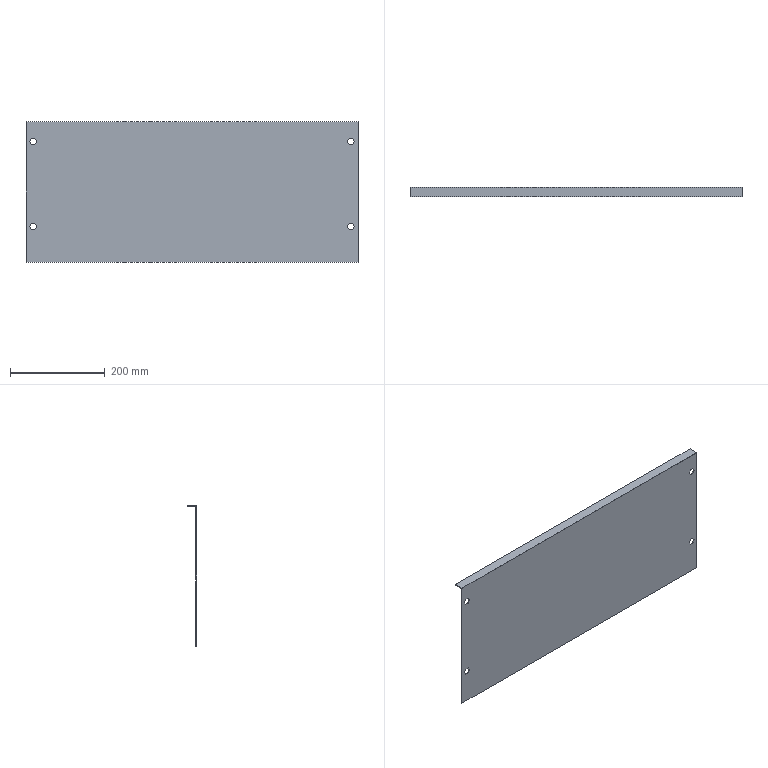Part | SolidWorks | features BaseBody 1 | 1 solid | 32 faces | box 700 x 20 x 297 mm | volume 439829 mm3 | plane 32
STEP:
#1=CARTESIAN_POINT('',(896.946,-3640.973,118.471));
#2=VERTEX_POINT('',#1);
#3=CARTESIAN_POINT('',(896.946,-3640.973,415.471));
#4=VERTEX_POINT('',#3);
#5=CARTESIAN_POINT('',(896.946,-3640.973,415.471));
#6=DIRECTION('',(0.,0.,1.));
#7=VECTOR('',#6,1000.);
#8=LINE('',#5,#7);
#9=EDGE_CURVE('',#2,#4,#8,.T.);
#10=ORIENTED_EDGE('',*,*,#9,.T.);
#11=CARTESIAN_POINT('',(196.946,-3640.973,415.471));
#12=VERTEX_POINT('',#11);
#13=CARTESIAN_POINT('',(896.946,-3640.973,415.471));
#14=DIRECTION('',(-1.,0.,0.));
#15=VECTOR('',#14,1000.);
#16=LINE('',#13,#15);
#17=EDGE_CURVE('',#4,#12,#16,.T.);
#18=ORIENTED_EDGE('',*,*,#17,.T.);
#19=CARTESIAN_POINT('',(196.946,-3640.973,118.471));
#20=VERTEX_POINT('',#19);
#21=CARTESIAN_POINT('',(196.946,-3640.973,415.471));
#22=DIRECTION('',(0.,0.,-1.));
#23=VECTOR('',#22,1000.);
#24=LINE('',#21,#23);
#25=EDGE_CURVE('',#12,#20,#24,.T.);
#26=ORIENTED_EDGE('',*,*,#25,.T.);
#27=CARTESIAN_POINT('',(896.946,-3640.973,118.471));
#28=DIRECTION('',(1.,0.,0.));
#29=VECTOR('',#28,1000.);
#30=LINE('',#27,#29);
#31=EDGE_CURVE('',#20,#2,#30,.T.);
#32=ORIENTED_EDGE('',*,*,#31,.T.);
#33=EDGE_LOOP('',(#10,#18,#26,#32));
#34=FACE_OUTER_BOUND('',#33,.T.);
#35=CARTESIAN_POINT('',(878.193,-3640.973,367.471));
#36=VERTEX_POINT('',#35);
#37=CARTESIAN_POINT('',(874.44,-3640.973,373.971));
#38=VERTEX_POINT('',#37);
#39=CARTESIAN_POINT('',(878.193,-3640.973,367.471));
#40=DIRECTION('',(-0.5,0.,0.866));
#41=VECTOR('',#40,1000.);
#42=LINE('',#39,#41);
#43=EDGE_CURVE('',#36,#38,#42,.T.);
#44=ORIENTED_EDGE('',*,*,#43,.T.);
#45=CARTESIAN_POINT('',(878.193,-3640.973,380.471));
#46=VERTEX_POINT('',#45);
#47=CARTESIAN_POINT('',(874.44,-3640.973,373.971));
#48=DIRECTION('',(0.5,0.,0.866));
#49=VECTOR('',#48,1000.);
#50=LINE('',#47,#49);
#51=EDGE_CURVE('',#38,#46,#50,.T.);
#52=ORIENTED_EDGE('',*,*,#51,.T.);
#53=CARTESIAN_POINT('',(885.698,-3640.973,380.471));
#54=VERTEX_POINT('',#53);
#55=CARTESIAN_POINT('',(896.946,-3640.973,380.471));
#56=DIRECTION('',(1.,0.,0.));
#57=VECTOR('',#56,1000.);
#58=LINE('',#55,#57);
#59=EDGE_CURVE('',#46,#54,#58,.T.);
#60=ORIENTED_EDGE('',*,*,#59,.T.);
#61=CARTESIAN_POINT('',(889.451,-3640.973,373.971));
#62=VERTEX_POINT('',#61);
#63=CARTESIAN_POINT('',(885.698,-3640.973,380.471));
#64=DIRECTION('',(0.5,0.,-0.866));
#65=VECTOR('',#64,1000.);
#66=LINE('',#63,#65);
#67=EDGE_CURVE('',#54,#62,#66,.T.);
#68=ORIENTED_EDGE('',*,*,#67,.T.);
#69=CARTESIAN_POINT('',(885.698,-3640.973,367.471));
#70=VERTEX_POINT('',#69);
#71=CARTESIAN_POINT('',(889.451,-3640.973,373.971));
#72=DIRECTION('',(-0.5,0.,-0.866));
#73=VECTOR('',#72,1000.);
#74=LINE('',#71,#73);
#75=EDGE_CURVE('',#62,#70,#74,.T.);
#76=ORIENTED_EDGE('',*,*,#75,.T.);
#77=CARTESIAN_POINT('',(896.946,-3640.973,367.471));
#78=DIRECTION('',(-1.,0.,0.));
#79=VECTOR('',#78,1000.);
#80=LINE('',#77,#79);
#81=EDGE_CURVE('',#70,#36,#80,.T.);
#82=ORIENTED_EDGE('',*,*,#81,.T.);
#83=EDGE_LOOP('',(#44,#52,#60,#68,#76,#82));
#84=FACE_BOUND('',#83,.T.);
#85=CARTESIAN_POINT('',(208.193,-3640.973,187.471));
#86=VERTEX_POINT('',#85);
#87=CARTESIAN_POINT('',(204.44,-3640.973,193.971));
#88=VERTEX_POINT('',#87);
#89=CARTESIAN_POINT('',(208.193,-3640.973,187.471));
#90=DIRECTION('',(-0.5,0.,0.866));
#91=VECTOR('',#90,1000.);
#92=LINE('',#89,#91);
#93=EDGE_CURVE('',#86,#88,#92,.T.);
#94=ORIENTED_EDGE('',*,*,#93,.T.);
#95=CARTESIAN_POINT('',(208.193,-3640.973,200.471));
#96=VERTEX_POINT('',#95);
#97=CARTESIAN_POINT('',(204.44,-3640.973,193.971));
#98=DIRECTION('',(0.5,0.,0.866));
#99=VECTOR('',#98,1000.);
#100=LINE('',#97,#99);
#101=EDGE_CURVE('',#88,#96,#100,.T.);
#102=ORIENTED_EDGE('',*,*,#101,.T.);
#103=CARTESIAN_POINT('',(215.698,-3640.973,200.471));
#104=VERTEX_POINT('',#103);
#105=CARTESIAN_POINT('',(896.946,-3640.973,200.471));
#106=DIRECTION('',(1.,0.,0.));
#107=VECTOR('',#106,1000.);
#108=LINE('',#105,#107);
#109=EDGE_CURVE('',#96,#104,#108,.T.);
#110=ORIENTED_EDGE('',*,*,#109,.T.);
#111=CARTESIAN_POINT('',(219.451,-3640.973,193.971));
#112=VERTEX_POINT('',#111);
#113=CARTESIAN_POINT('',(215.698,-3640.973,200.471));
#114=DIRECTION('',(0.5,0.,-0.866));
#115=VECTOR('',#114,1000.);
#116=LINE('',#113,#115);
#117=EDGE_CURVE('',#104,#112,#116,.T.);
#118=ORIENTED_EDGE('',*,*,#117,.T.);
#119=CARTESIAN_POINT('',(215.698,-3640.973,187.471));
#120=VERTEX_POINT('',#119);
#121=CARTESIAN_POINT('',(219.451,-3640.973,193.971));
#122=DIRECTION('',(-0.5,0.,-0.866));
#123=VECTOR('',#122,1000.);
#124=LINE('',#121,#123);
#125=EDGE_CURVE('',#112,#120,#124,.T.);
#126=ORIENTED_EDGE('',*,*,#125,.T.);
#127=CARTESIAN_POINT('',(896.946,-3640.973,187.471));
#128=DIRECTION('',(-1.,0.,0.));
#129=VECTOR('',#128,1000.);
#130=LINE('',#127,#129);
#131=EDGE_CURVE('',#120,#86,#130,.T.);
#132=ORIENTED_EDGE('',*,*,#131,.T.);
#133=EDGE_LOOP('',(#94,#102,#110,#118,#126,#132));
#134=FACE_BOUND('',#133,.T.);
#135=CARTESIAN_POINT('',(208.193,-3640.973,367.471));
#136=VERTEX_POINT('',#135);
#137=CARTESIAN_POINT('',(204.44,-3640.973,373.971));
#138=VERTEX_POINT('',#137);
#139=CARTESIAN_POINT('',(208.193,-3640.973,367.471));
#140=DIRECTION('',(-0.5,0.,0.866));
#141=VECTOR('',#140,1000.);
#142=LINE('',#139,#141);
#143=EDGE_CURVE('',#136,#138,#142,.T.);
#144=ORIENTED_EDGE('',*,*,#143,.T.);
#145=CARTESIAN_POINT('',(208.193,-3640.973,380.471));
#146=VERTEX_POINT('',#145);
#147=CARTESIAN_POINT('',(204.44,-3640.973,373.971));
#148=DIRECTION('',(0.5,0.,0.866));
#149=VECTOR('',#148,1000.);
#150=LINE('',#147,#149);
#151=EDGE_CURVE('',#138,#146,#150,.T.);
#152=ORIENTED_EDGE('',*,*,#151,.T.);
#153=CARTESIAN_POINT('',(215.698,-3640.973,380.471));
#154=VERTEX_POINT('',#153);
#155=CARTESIAN_POINT('',(896.946,-3640.973,380.471));
#156=DIRECTION('',(1.,0.,0.));
#157=VECTOR('',#156,1000.);
#158=LINE('',#155,#157);
#159=EDGE_CURVE('',#146,#154,#158,.T.);
#160=ORIENTED_EDGE('',*,*,#159,.T.);
#161=CARTESIAN_POINT('',(219.451,-3640.973,373.971));
#162=VERTEX_POINT('',#161);
#163=CARTESIAN_POINT('',(215.698,-3640.973,380.471));
#164=DIRECTION('',(0.5,0.,-0.866));
#165=VECTOR('',#164,1000.);
#166=LINE('',#163,#165);
#167=EDGE_CURVE('',#154,#162,#166,.T.);
#168=ORIENTED_EDGE('',*,*,#167,.T.);
#169=CARTESIAN_POINT('',(215.698,-3640.973,367.471));
#170=VERTEX_POINT('',#169);
#171=CARTESIAN_POINT('',(219.451,-3640.973,373.971));
#172=DIRECTION('',(-0.5,0.,-0.866));
#173=VECTOR('',#172,1000.);
#174=LINE('',#171,#173);
#175=EDGE_CURVE('',#162,#170,#174,.T.);
#176=ORIENTED_EDGE('',*,*,#175,.T.);
#177=CARTESIAN_POINT('',(896.946,-3640.973,367.471));
#178=DIRECTION('',(-1.,0.,0.));
#179=VECTOR('',#178,1000.);
#180=LINE('',#177,#179);
#181=EDGE_CURVE('',#170,#136,#180,.T.);
#182=ORIENTED_EDGE('',*,*,#181,.T.);
#183=EDGE_LOOP('',(#144,#152,#160,#168,#176,#182));
#184=FACE_BOUND('',#183,.T.);
#185=CARTESIAN_POINT('',(878.193,-3640.973,187.471));
#186=VERTEX_POINT('',#185);
#187=CARTESIAN_POINT('',(874.44,-3640.973,193.971));
#188=VERTEX_POINT('',#187);
#189=CARTESIAN_POINT('',(878.193,-3640.973,187.471));
#190=DIRECTION('',(-0.5,0.,0.866));
#191=VECTOR('',#190,1000.);
#192=LINE('',#189,#191);
#193=EDGE_CURVE('',#186,#188,#192,.T.);
#194=ORIENTED_EDGE('',*,*,#193,.T.);
#195=CARTESIAN_POINT('',(878.193,-3640.973,200.471));
#196=VERTEX_POINT('',#195);
#197=CARTESIAN_POINT('',(874.44,-3640.973,193.971));
#198=DIRECTION('',(0.5,0.,0.866));
#199=VECTOR('',#198,1000.);
#200=LINE('',#197,#199);
#201=EDGE_CURVE('',#188,#196,#200,.T.);
#202=ORIENTED_EDGE('',*,*,#201,.T.);
#203=CARTESIAN_POINT('',(885.698,-3640.973,200.471));
#204=VERTEX_POINT('',#203);
#205=CARTESIAN_POINT('',(896.946,-3640.973,200.471));
#206=DIRECTION('',(1.,0.,0.));
#207=VECTOR('',#206,1000.);
#208=LINE('',#205,#207);
#209=EDGE_CURVE('',#196,#204,#208,.T.);
#210=ORIENTED_EDGE('',*,*,#209,.T.);
#211=CARTESIAN_POINT('',(889.451,-3640.973,193.971));
#212=VERTEX_POINT('',#211);
#213=CARTESIAN_POINT('',(885.698,-3640.973,200.471));
#214=DIRECTION('',(0.5,0.,-0.866));
#215=VECTOR('',#214,1000.);
#216=LINE('',#213,#215);
#217=EDGE_CURVE('',#204,#212,#216,.T.);
#218=ORIENTED_EDGE('',*,*,#217,.T.);
#219=CARTESIAN_POINT('',(885.698,-3640.973,187.471));
#220=VERTEX_POINT('',#219);
#221=CARTESIAN_POINT('',(889.451,-3640.973,193.971));
#222=DIRECTION('',(-0.5,0.,-0.866));
#223=VECTOR('',#222,1000.);
#224=LINE('',#221,#223);
#225=EDGE_CURVE('',#212,#220,#224,.T.);
#226=ORIENTED_EDGE('',*,*,#225,.T.);
#227=CARTESIAN_POINT('',(896.946,-3640.973,187.471));
#228=DIRECTION('',(-1.,0.,0.));
#229=VECTOR('',#228,1000.);
#230=LINE('',#227,#229);
#231=EDGE_CURVE('',#220,#186,#230,.T.);
#232=ORIENTED_EDGE('',*,*,#231,.T.);
#233=EDGE_LOOP('',(#194,#202,#210,#218,#226,#232));
#234=FACE_BOUND('',#233,.T.);
#235=CARTESIAN_POINT('',(896.946,-3640.973,415.471));
#236=DIRECTION('',(0.,-1.,0.));
#237=DIRECTION('',(0.,0.,-1.));
#238=AXIS2_PLACEMENT_3D('',#235,#236,#237);
#239=PLANE('',#238);
#240=ADVANCED_FACE('',(#34,#84,#134,#184,#234),#239,.T.);
#241=CARTESIAN_POINT('',(896.946,-3620.973,415.471));
#242=VERTEX_POINT('',#241);
#243=CARTESIAN_POINT('',(896.946,-3620.973,415.471));
#244=DIRECTION('',(0.,1.,0.));
#245=VECTOR('',#244,1000.);
#246=LINE('',#243,#245);
#247=EDGE_CURVE('',#4,#242,#246,.T.);
#248=ORIENTED_EDGE('',*,*,#247,.T.);
#249=CARTESIAN_POINT('',(196.946,-3620.973,415.471));
#250=VERTEX_POINT('',#249);
#251=CARTESIAN_POINT('',(896.946,-3620.973,415.471));
#252=DIRECTION('',(-1.,0.,0.));
#253=VECTOR('',#252,1000.);
#254=LINE('',#251,#253);
#255=EDGE_CURVE('',#242,#250,#254,.T.);
#256=ORIENTED_EDGE('',*,*,#255,.T.);
#257=CARTESIAN_POINT('',(196.946,-3620.973,415.471));
#258=DIRECTION('',(0.,-1.,0.));
#259=VECTOR('',#258,1000.);
#260=LINE('',#257,#259);
#261=EDGE_CURVE('',#250,#12,#260,.T.);
#262=ORIENTED_EDGE('',*,*,#261,.T.);
#263=ORIENTED_EDGE('',*,*,#17,.F.);
#264=EDGE_LOOP('',(#248,#256,#262,#263));
#265=FACE_OUTER_BOUND('',#264,.T.);
#266=CARTESIAN_POINT('',(896.946,-3620.973,415.471));
#267=DIRECTION('',(0.,0.,1.));
#268=DIRECTION('',(1.,0.,0.));
#269=AXIS2_PLACEMENT_3D('',#266,#267,#268);
#270=PLANE('',#269);
#271=ADVANCED_FACE('',(#265),#270,.T.);
#272=ORIENTED_EDGE('',*,*,#247,.F.);
#273=ORIENTED_EDGE('',*,*,#9,.F.);
#274=CARTESIAN_POINT('',(896.946,-3638.973,118.471));
#275=VERTEX_POINT('',#274);
#276=CARTESIAN_POINT('',(896.946,-3639.349,118.471));
#277=DIRECTION('',(0.,1.,0.));
#278=VECTOR('',#277,1000.);
#279=LINE('',#276,#278);
#280=EDGE_CURVE('',#2,#275,#279,.T.);
#281=ORIENTED_EDGE('',*,*,#280,.T.);
#282=CARTESIAN_POINT('',(896.946,-3638.973,413.471));
#283=VERTEX_POINT('',#282);
#284=CARTESIAN_POINT('',(896.946,-3638.973,275.347));
#285=DIRECTION('',(0.,0.,1.));
#286=VECTOR('',#285,1000.);
#287=LINE('',#284,#286);
#288=EDGE_CURVE('',#275,#283,#287,.T.);
#289=ORIENTED_EDGE('',*,*,#288,.T.);
#290=CARTESIAN_POINT('',(896.946,-3620.973,413.471));
#291=VERTEX_POINT('',#290);
#292=CARTESIAN_POINT('',(896.946,-3639.349,413.471));
#293=DIRECTION('',(0.,1.,0.));
#294=VECTOR('',#293,1000.);
#295=LINE('',#292,#294);
#296=EDGE_CURVE('',#283,#291,#295,.T.);
#297=ORIENTED_EDGE('',*,*,#296,.T.);
#298=CARTESIAN_POINT('',(896.946,-3620.973,275.347));
#299=DIRECTION('',(0.,0.,1.));
#300=VECTOR('',#299,1000.);
#301=LINE('',#298,#300);
#302=EDGE_CURVE('',#291,#242,#301,.T.);
#303=ORIENTED_EDGE('',*,*,#302,.T.);
#304=EDGE_LOOP('',(#272,#273,#281,#289,#297,#303));
#305=FACE_OUTER_BOUND('',#304,.T.);
#306=CARTESIAN_POINT('',(896.946,-3639.349,275.347));
#307=DIRECTION('',(1.,0.,0.));
#308=DIRECTION('',(0.,0.,-1.));
#309=AXIS2_PLACEMENT_3D('',#306,#307,#308);
#310=PLANE('',#309);
#311=ADVANCED_FACE('',(#305),#310,.T.);
#312=ORIENTED_EDGE('',*,*,#280,.F.);
#313=ORIENTED_EDGE('',*,*,#31,.F.);
#314=CARTESIAN_POINT('',(196.946,-3638.973,118.471));
#315=VERTEX_POINT('',#314);
#316=CARTESIAN_POINT('',(196.946,-3640.973,118.471));
#317=DIRECTION('',(0.,1.,0.));
#318=VECTOR('',#317,1000.);
#319=LINE('',#316,#318);
#320=EDGE_CURVE('',#20,#315,#319,.T.);
#321=ORIENTED_EDGE('',*,*,#320,.T.);
#322=CARTESIAN_POINT('',(896.946,-3638.973,118.471));
#323=DIRECTION('',(1.,0.,0.));
#324=VECTOR('',#323,1000.);
#325=LINE('',#322,#324);
#326=EDGE_CURVE('',#315,#275,#325,.T.);
#327=ORIENTED_EDGE('',*,*,#326,.T.);
#328=EDGE_LOOP('',(#312,#313,#321,#327));
#329=FACE_OUTER_BOUND('',#328,.T.);
#330=CARTESIAN_POINT('',(896.946,-3640.973,118.471));
#331=DIRECTION('',(0.,0.,-1.));
#332=DIRECTION('',(-1.,0.,0.));
#333=AXIS2_PLACEMENT_3D('',#330,#331,#332);
#334=PLANE('',#333);
#335=ADVANCED_FACE('',(#329),#334,.T.);
#336=ORIENTED_EDGE('',*,*,#320,.F.);
#337=ORIENTED_EDGE('',*,*,#25,.F.);
#338=ORIENTED_EDGE('',*,*,#261,.F.);
#339=CARTESIAN_POINT('',(196.946,-3620.973,413.471));
#340=VERTEX_POINT('',#339);
#341=CARTESIAN_POINT('',(196.946,-3620.973,275.347));
#342=DIRECTION('',(0.,0.,1.));
#343=VECTOR('',#342,1000.);
#344=LINE('',#341,#343);
#345=EDGE_CURVE('',#340,#250,#344,.T.);
#346=ORIENTED_EDGE('',*,*,#345,.F.);
#347=CARTESIAN_POINT('',(196.946,-3638.973,413.471));
#348=VERTEX_POINT('',#347);
#349=CARTESIAN_POINT('',(196.946,-3639.349,413.471));
#350=DIRECTION('',(0.,1.,0.));
#351=VECTOR('',#350,1000.);
#352=LINE('',#349,#351);
#353=EDGE_CURVE('',#348,#340,#352,.T.);
#354=ORIENTED_EDGE('',*,*,#353,.F.);
#355=CARTESIAN_POINT('',(196.946,-3638.973,275.347));
#356=DIRECTION('',(0.,0.,1.));
#357=VECTOR('',#356,1000.);
#358=LINE('',#355,#357);
#359=EDGE_CURVE('',#315,#348,#358,.T.);
#360=ORIENTED_EDGE('',*,*,#359,.F.);
#361=EDGE_LOOP('',(#336,#337,#338,#346,#354,#360));
#362=FACE_OUTER_BOUND('',#361,.T.);
#363=CARTESIAN_POINT('',(196.946,-3639.349,275.347));
#364=DIRECTION('',(1.,0.,0.));
#365=DIRECTION('',(0.,0.,-1.));
#366=AXIS2_PLACEMENT_3D('',#363,#364,#365);
#367=PLANE('',#366);
#368=ADVANCED_FACE('',(#362),#367,.F.);
#369=CARTESIAN_POINT('',(878.193,-3638.973,380.471));
#370=VERTEX_POINT('',#369);
#371=CARTESIAN_POINT('',(878.193,-3446.271,380.471));
#372=DIRECTION('',(0.,1.,0.));
#373=VECTOR('',#372,1000.);
#374=LINE('',#371,#373);
#375=EDGE_CURVE('',#46,#370,#374,.T.);
#376=ORIENTED_EDGE('',*,*,#375,.F.);
#377=ORIENTED_EDGE('',*,*,#51,.F.);
#378=CARTESIAN_POINT('',(874.44,-3638.973,373.971));
#379=VERTEX_POINT('',#378);
#380=CARTESIAN_POINT('',(874.44,-3446.271,373.971));
#381=DIRECTION('',(0.,-1.,0.));
#382=VECTOR('',#381,1000.);
#383=LINE('',#380,#382);
#384=EDGE_CURVE('',#379,#38,#383,.T.);
#385=ORIENTED_EDGE('',*,*,#384,.F.);
#386=CARTESIAN_POINT('',(878.193,-3638.973,380.471));
#387=DIRECTION('',(-0.5,0.,-0.866));
#388=VECTOR('',#387,1000.);
#389=LINE('',#386,#388);
#390=EDGE_CURVE('',#370,#379,#389,.T.);
#391=ORIENTED_EDGE('',*,*,#390,.F.);
#392=EDGE_LOOP('',(#376,#377,#385,#391));
#393=FACE_OUTER_BOUND('',#392,.T.);
#394=CARTESIAN_POINT('',(878.193,-3446.271,380.471));
#395=DIRECTION('',(-0.866,0.,0.5));
#396=DIRECTION('',(0.5,0.,0.866));
#397=AXIS2_PLACEMENT_3D('',#394,#395,#396);
#398=PLANE('',#397);
#399=ADVANCED_FACE('',(#393),#398,.F.);
#400=ORIENTED_EDGE('',*,*,#384,.T.);
#401=ORIENTED_EDGE('',*,*,#43,.F.);
#402=CARTESIAN_POINT('',(878.193,-3638.973,367.471));
#403=VERTEX_POINT('',#402);
#404=CARTESIAN_POINT('',(878.193,-3446.271,367.471));
#405=DIRECTION('',(0.,-1.,0.));
#406=VECTOR('',#405,1000.);
#407=LINE('',#404,#406);
#408=EDGE_CURVE('',#403,#36,#407,.T.);
#409=ORIENTED_EDGE('',*,*,#408,.F.);
#410=CARTESIAN_POINT('',(874.44,-3638.973,373.971));
#411=DIRECTION('',(0.5,0.,-0.866));
#412=VECTOR('',#411,1000.);
#413=LINE('',#410,#412);
#414=EDGE_CURVE('',#379,#403,#413,.T.);
#415=ORIENTED_EDGE('',*,*,#414,.F.);
#416=EDGE_LOOP('',(#400,#401,#409,#415));
#417=FACE_OUTER_BOUND('',#416,.T.);
#418=CARTESIAN_POINT('',(874.44,-3446.271,373.971));
#419=DIRECTION('',(-0.866,0.,-0.5));
#420=DIRECTION('',(-0.5,0.,0.866));
#421=AXIS2_PLACEMENT_3D('',#418,#419,#420);
#422=PLANE('',#421);
#423=ADVANCED_FACE('',(#417),#422,.F.);
#424=ORIENTED_EDGE('',*,*,#408,.T.);
#425=ORIENTED_EDGE('',*,*,#81,.F.);
#426=CARTESIAN_POINT('',(885.698,-3638.973,367.471));
#427=VERTEX_POINT('',#426);
#428=CARTESIAN_POINT('',(885.698,-3446.271,367.471));
#429=DIRECTION('',(0.,-1.,0.));
#430=VECTOR('',#429,1000.);
#431=LINE('',#428,#430);
#432=EDGE_CURVE('',#427,#70,#431,.T.);
#433=ORIENTED_EDGE('',*,*,#432,.F.);
#434=CARTESIAN_POINT('',(878.193,-3638.973,367.471));
#435=DIRECTION('',(1.,0.,0.));
#436=VECTOR('',#435,1000.);
#437=LINE('',#434,#436);
#438=EDGE_CURVE('',#403,#427,#437,.T.);
#439=ORIENTED_EDGE('',*,*,#438,.F.);
#440=EDGE_LOOP('',(#424,#425,#433,#439));
#441=FACE_OUTER_BOUND('',#440,.T.);
#442=CARTESIAN_POINT('',(878.193,-3446.271,367.471));
#443=DIRECTION('',(0.,0.,-1.));
#444=DIRECTION('',(-1.,0.,0.));
#445=AXIS2_PLACEMENT_3D('',#442,#443,#444);
#446=PLANE('',#445);
#447=ADVANCED_FACE('',(#441),#446,.F.);
#448=ORIENTED_EDGE('',*,*,#432,.T.);
#449=ORIENTED_EDGE('',*,*,#75,.F.);
#450=CARTESIAN_POINT('',(889.451,-3638.973,373.971));
#451=VERTEX_POINT('',#450);
#452=CARTESIAN_POINT('',(889.451,-3446.271,373.971));
#453=DIRECTION('',(0.,-1.,0.));
#454=VECTOR('',#453,1000.);
#455=LINE('',#452,#454);
#456=EDGE_CURVE('',#451,#62,#455,.T.);
#457=ORIENTED_EDGE('',*,*,#456,.F.);
#458=CARTESIAN_POINT('',(885.698,-3638.973,367.471));
#459=DIRECTION('',(0.5,0.,0.866));
#460=VECTOR('',#459,1000.);
#461=LINE('',#458,#460);
#462=EDGE_CURVE('',#427,#451,#461,.T.);
#463=ORIENTED_EDGE('',*,*,#462,.F.);
#464=EDGE_LOOP('',(#448,#449,#457,#463));
#465=FACE_OUTER_BOUND('',#464,.T.);
#466=CARTESIAN_POINT('',(885.698,-3446.271,367.471));
#467=DIRECTION('',(0.866,0.,-0.5));
#468=DIRECTION('',(-0.5,0.,-0.866));
#469=AXIS2_PLACEMENT_3D('',#466,#467,#468);
#470=PLANE('',#469);
#471=ADVANCED_FACE('',(#465),#470,.F.);
#472=ORIENTED_EDGE('',*,*,#456,.T.);
#473=ORIENTED_EDGE('',*,*,#67,.F.);
#474=CARTESIAN_POINT('',(885.698,-3638.973,380.471));
#475=VERTEX_POINT('',#474);
#476=CARTESIAN_POINT('',(885.698,-3446.271,380.471));
#477=DIRECTION('',(0.,-1.,0.));
#478=VECTOR('',#477,1000.);
#479=LINE('',#476,#478);
#480=EDGE_CURVE('',#475,#54,#479,.T.);
#481=ORIENTED_EDGE('',*,*,#480,.F.);
#482=CARTESIAN_POINT('',(889.451,-3638.973,373.971));
#483=DIRECTION('',(-0.5,0.,0.866));
#484=VECTOR('',#483,1000.);
#485=LINE('',#482,#484);
#486=EDGE_CURVE('',#451,#475,#485,.T.);
#487=ORIENTED_EDGE('',*,*,#486,.F.);
#488=EDGE_LOOP('',(#472,#473,#481,#487));
#489=FACE_OUTER_BOUND('',#488,.T.);
#490=CARTESIAN_POINT('',(889.451,-3446.271,373.971));
#491=DIRECTION('',(0.866,0.,0.5));
#492=DIRECTION('',(0.5,0.,-0.866));
#493=AXIS2_PLACEMENT_3D('',#490,#491,#492);
#494=PLANE('',#493);
#495=ADVANCED_FACE('',(#489),#494,.F.);
#496=ORIENTED_EDGE('',*,*,#480,.T.);
#497=ORIENTED_EDGE('',*,*,#59,.F.);
#498=ORIENTED_EDGE('',*,*,#375,.T.);
#499=CARTESIAN_POINT('',(885.698,-3638.973,380.471));
#500=DIRECTION('',(-1.,0.,0.));
#501=VECTOR('',#500,1000.);
#502=LINE('',#499,#501);
#503=EDGE_CURVE('',#475,#370,#502,.T.);
#504=ORIENTED_EDGE('',*,*,#503,.F.);
#505=EDGE_LOOP('',(#496,#497,#498,#504));
#506=FACE_OUTER_BOUND('',#505,.T.);
#507=CARTESIAN_POINT('',(885.698,-3446.271,380.471));
#508=DIRECTION('',(0.,0.,1.));
#509=DIRECTION('',(1.,0.,0.));
#510=AXIS2_PLACEMENT_3D('',#507,#508,#509);
#511=PLANE('',#510);
#512=ADVANCED_FACE('',(#506),#511,.F.);
#513=CARTESIAN_POINT('',(208.193,-3638.973,200.471));
#514=VERTEX_POINT('',#513);
#515=CARTESIAN_POINT('',(208.193,-3446.271,200.471));
#516=DIRECTION('',(0.,1.,0.));
#517=VECTOR('',#516,1000.);
#518=LINE('',#515,#517);
#519=EDGE_CURVE('',#96,#514,#518,.T.);
#520=ORIENTED_EDGE('',*,*,#519,.F.);
#521=ORIENTED_EDGE('',*,*,#101,.F.);
#522=CARTESIAN_POINT('',(204.44,-3638.973,193.971));
#523=VERTEX_POINT('',#522);
#524=CARTESIAN_POINT('',(204.44,-3446.271,193.971));
#525=DIRECTION('',(0.,-1.,0.));
#526=VECTOR('',#525,1000.);
#527=LINE('',#524,#526);
#528=EDGE_CURVE('',#523,#88,#527,.T.);
#529=ORIENTED_EDGE('',*,*,#528,.F.);
#530=CARTESIAN_POINT('',(204.44,-3638.973,193.971));
#531=DIRECTION('',(-0.5,0.,-0.866));
#532=VECTOR('',#531,1000.);
#533=LINE('',#530,#532);
#534=EDGE_CURVE('',#514,#523,#533,.T.);
#535=ORIENTED_EDGE('',*,*,#534,.F.);
#536=EDGE_LOOP('',(#520,#521,#529,#535));
#537=FACE_OUTER_BOUND('',#536,.T.);
#538=CARTESIAN_POINT('',(204.44,-3446.271,193.971));
#539=DIRECTION('',(-0.866,0.,0.5));
#540=DIRECTION('',(0.5,0.,0.866));
#541=AXIS2_PLACEMENT_3D('',#538,#539,#540);
#542=PLANE('',#541);
#543=ADVANCED_FACE('',(#537),#542,.F.);
#544=ORIENTED_EDGE('',*,*,#528,.T.);
#545=ORIENTED_EDGE('',*,*,#93,.F.);
#546=CARTESIAN_POINT('',(208.193,-3638.973,187.471));
#547=VERTEX_POINT('',#546);
#548=CARTESIAN_POINT('',(208.193,-3446.271,187.471));
#549=DIRECTION('',(0.,-1.,0.));
#550=VECTOR('',#549,1000.);
#551=LINE('',#548,#550);
#552=EDGE_CURVE('',#547,#86,#551,.T.);
#553=ORIENTED_EDGE('',*,*,#552,.F.);
#554=CARTESIAN_POINT('',(208.193,-3638.973,187.471));
#555=DIRECTION('',(0.5,0.,-0.866));
#556=VECTOR('',#555,1000.);
#557=LINE('',#554,#556);
#558=EDGE_CURVE('',#523,#547,#557,.T.);
#559=ORIENTED_EDGE('',*,*,#558,.F.);
#560=EDGE_LOOP('',(#544,#545,#553,#559));
#561=FACE_OUTER_BOUND('',#560,.T.);
#562=CARTESIAN_POINT('',(208.193,-3446.271,187.471));
#563=DIRECTION('',(-0.866,0.,-0.5));
#564=DIRECTION('',(-0.5,0.,0.866));
#565=AXIS2_PLACEMENT_3D('',#562,#563,#564);
#566=PLANE('',#565);
#567=ADVANCED_FACE('',(#561),#566,.F.);
#568=ORIENTED_EDGE('',*,*,#552,.T.);
#569=ORIENTED_EDGE('',*,*,#131,.F.);
#570=CARTESIAN_POINT('',(215.698,-3638.973,187.471));
#571=VERTEX_POINT('',#570);
#572=CARTESIAN_POINT('',(215.698,-3446.271,187.471));
#573=DIRECTION('',(0.,-1.,0.));
#574=VECTOR('',#573,1000.);
#575=LINE('',#572,#574);
#576=EDGE_CURVE('',#571,#120,#575,.T.);
#577=ORIENTED_EDGE('',*,*,#576,.F.);
#578=CARTESIAN_POINT('',(215.698,-3638.973,187.471));
#579=DIRECTION('',(1.,0.,0.));
#580=VECTOR('',#579,1000.);
#581=LINE('',#578,#580);
#582=EDGE_CURVE('',#547,#571,#581,.T.);
#583=ORIENTED_EDGE('',*,*,#582,.F.);
#584=EDGE_LOOP('',(#568,#569,#577,#583));
#585=FACE_OUTER_BOUND('',#584,.T.);
#586=CARTESIAN_POINT('',(215.698,-3446.271,187.471));
#587=DIRECTION('',(0.,0.,-1.));
#588=DIRECTION('',(-1.,0.,0.));
#589=AXIS2_PLACEMENT_3D('',#586,#587,#588);
#590=PLANE('',#589);
#591=ADVANCED_FACE('',(#585),#590,.F.);
#592=ORIENTED_EDGE('',*,*,#576,.T.);
#593=ORIENTED_EDGE('',*,*,#125,.F.);
#594=CARTESIAN_POINT('',(219.451,-3638.973,193.971));
#595=VERTEX_POINT('',#594);
#596=CARTESIAN_POINT('',(219.451,-3446.271,193.971));
#597=DIRECTION('',(0.,-1.,0.));
#598=VECTOR('',#597,1000.);
#599=LINE('',#596,#598);
#600=EDGE_CURVE('',#595,#112,#599,.T.);
#601=ORIENTED_EDGE('',*,*,#600,.F.);
#602=CARTESIAN_POINT('',(219.451,-3638.973,193.971));
#603=DIRECTION('',(0.5,0.,0.866));
#604=VECTOR('',#603,1000.);
#605=LINE('',#602,#604);
#606=EDGE_CURVE('',#571,#595,#605,.T.);
#607=ORIENTED_EDGE('',*,*,#606,.F.);
#608=EDGE_LOOP('',(#592,#593,#601,#607));
#609=FACE_OUTER_BOUND('',#608,.T.);
#610=CARTESIAN_POINT('',(219.451,-3446.271,193.971));
#611=DIRECTION('',(0.866,0.,-0.5));
#612=DIRECTION('',(-0.5,0.,-0.866));
#613=AXIS2_PLACEMENT_3D('',#610,#611,#612);
#614=PLANE('',#613);
#615=ADVANCED_FACE('',(#609),#614,.F.);
#616=ORIENTED_EDGE('',*,*,#600,.T.);
#617=ORIENTED_EDGE('',*,*,#117,.F.);
#618=CARTESIAN_POINT('',(215.698,-3638.973,200.471));
#619=VERTEX_POINT('',#618);
#620=CARTESIAN_POINT('',(215.698,-3446.271,200.471));
#621=DIRECTION('',(0.,-1.,0.));
#622=VECTOR('',#621,1000.);
#623=LINE('',#620,#622);
#624=EDGE_CURVE('',#619,#104,#623,.T.);
#625=ORIENTED_EDGE('',*,*,#624,.F.);
#626=CARTESIAN_POINT('',(215.698,-3638.973,200.471));
#627=DIRECTION('',(-0.5,0.,0.866));
#628=VECTOR('',#627,1000.);
#629=LINE('',#626,#628);
#630=EDGE_CURVE('',#595,#619,#629,.T.);
#631=ORIENTED_EDGE('',*,*,#630,.F.);
#632=EDGE_LOOP('',(#616,#617,#625,#631));
#633=FACE_OUTER_BOUND('',#632,.T.);
#634=CARTESIAN_POINT('',(215.698,-3446.271,200.471));
#635=DIRECTION('',(0.866,0.,0.5));
#636=DIRECTION('',(0.5,0.,-0.866));
#637=AXIS2_PLACEMENT_3D('',#634,#635,#636);
#638=PLANE('',#637);
#639=ADVANCED_FACE('',(#633),#638,.F.);
#640=ORIENTED_EDGE('',*,*,#624,.T.);
#641=ORIENTED_EDGE('',*,*,#109,.F.);
#642=ORIENTED_EDGE('',*,*,#519,.T.);
#643=CARTESIAN_POINT('',(208.193,-3638.973,200.471));
#644=DIRECTION('',(-1.,0.,0.));
#645=VECTOR('',#644,1000.);
#646=LINE('',#643,#645);
#647=EDGE_CURVE('',#619,#514,#646,.T.);
#648=ORIENTED_EDGE('',*,*,#647,.F.);
#649=EDGE_LOOP('',(#640,#641,#642,#648));
#650=FACE_OUTER_BOUND('',#649,.T.);
#651=CARTESIAN_POINT('',(208.193,-3446.271,200.471));
#652=DIRECTION('',(0.,0.,1.));
#653=DIRECTION('',(1.,0.,0.));
#654=AXIS2_PLACEMENT_3D('',#651,#652,#653);
#655=PLANE('',#654);
#656=ADVANCED_FACE('',(#650),#655,.F.);
#657=CARTESIAN_POINT('',(208.193,-3638.973,380.471));
#658=VERTEX_POINT('',#657);
#659=CARTESIAN_POINT('',(208.193,-3446.271,380.471));
#660=DIRECTION('',(0.,1.,0.));
#661=VECTOR('',#660,1000.);
#662=LINE('',#659,#661);
#663=EDGE_CURVE('',#146,#658,#662,.T.);
#664=ORIENTED_EDGE('',*,*,#663,.F.);
#665=ORIENTED_EDGE('',*,*,#151,.F.);
#666=CARTESIAN_POINT('',(204.44,-3638.973,373.971));
#667=VERTEX_POINT('',#666);
#668=CARTESIAN_POINT('',(204.44,-3446.271,373.971));
#669=DIRECTION('',(0.,-1.,0.));
#670=VECTOR('',#669,1000.);
#671=LINE('',#668,#670);
#672=EDGE_CURVE('',#667,#138,#671,.T.);
#673=ORIENTED_EDGE('',*,*,#672,.F.);
#674=CARTESIAN_POINT('',(204.44,-3638.973,373.971));
#675=DIRECTION('',(-0.5,0.,-0.866));
#676=VECTOR('',#675,1000.);
#677=LINE('',#674,#676);
#678=EDGE_CURVE('',#658,#667,#677,.T.);
#679=ORIENTED_EDGE('',*,*,#678,.F.);
#680=EDGE_LOOP('',(#664,#665,#673,#679));
#681=FACE_OUTER_BOUND('',#680,.T.);
#682=CARTESIAN_POINT('',(204.44,-3446.271,373.971));
#683=DIRECTION('',(-0.866,0.,0.5));
#684=DIRECTION('',(0.5,0.,0.866));
#685=AXIS2_PLACEMENT_3D('',#682,#683,#684);
#686=PLANE('',#685);
#687=ADVANCED_FACE('',(#681),#686,.F.);
#688=ORIENTED_EDGE('',*,*,#672,.T.);
#689=ORIENTED_EDGE('',*,*,#143,.F.);
#690=CARTESIAN_POINT('',(208.193,-3638.973,367.471));
#691=VERTEX_POINT('',#690);
#692=CARTESIAN_POINT('',(208.193,-3446.271,367.471));
#693=DIRECTION('',(0.,-1.,0.));
#694=VECTOR('',#693,1000.);
#695=LINE('',#692,#694);
#696=EDGE_CURVE('',#691,#136,#695,.T.);
#697=ORIENTED_EDGE('',*,*,#696,.F.);
#698=CARTESIAN_POINT('',(208.193,-3638.973,367.471));
#699=DIRECTION('',(0.5,0.,-0.866));
#700=VECTOR('',#699,1000.);
#701=LINE('',#698,#700);
#702=EDGE_CURVE('',#667,#691,#701,.T.);
#703=ORIENTED_EDGE('',*,*,#702,.F.);
#704=EDGE_LOOP('',(#688,#689,#697,#703));
#705=FACE_OUTER_BOUND('',#704,.T.);
#706=CARTESIAN_POINT('',(208.193,-3446.271,367.471));
#707=DIRECTION('',(-0.866,0.,-0.5));
#708=DIRECTION('',(-0.5,0.,0.866));
#709=AXIS2_PLACEMENT_3D('',#706,#707,#708);
#710=PLANE('',#709);
#711=ADVANCED_FACE('',(#705),#710,.F.);
#712=ORIENTED_EDGE('',*,*,#696,.T.);
#713=ORIENTED_EDGE('',*,*,#181,.F.);
#714=CARTESIAN_POINT('',(215.698,-3638.973,367.471));
#715=VERTEX_POINT('',#714);
#716=CARTESIAN_POINT('',(215.698,-3446.271,367.471));
#717=DIRECTION('',(0.,-1.,0.));
#718=VECTOR('',#717,1000.);
#719=LINE('',#716,#718);
#720=EDGE_CURVE('',#715,#170,#719,.T.);
#721=ORIENTED_EDGE('',*,*,#720,.F.);
#722=CARTESIAN_POINT('',(215.698,-3638.973,367.471));
#723=DIRECTION('',(1.,0.,0.));
#724=VECTOR('',#723,1000.);
#725=LINE('',#722,#724);
#726=EDGE_CURVE('',#691,#715,#725,.T.);
#727=ORIENTED_EDGE('',*,*,#726,.F.);
#728=EDGE_LOOP('',(#712,#713,#721,#727));
#729=FACE_OUTER_BOUND('',#728,.T.);
#730=CARTESIAN_POINT('',(215.698,-3446.271,367.471));
#731=DIRECTION('',(0.,0.,-1.));
#732=DIRECTION('',(-1.,0.,0.));
#733=AXIS2_PLACEMENT_3D('',#730,#731,#732);
#734=PLANE('',#733);
#735=ADVANCED_FACE('',(#729),#734,.F.);
#736=ORIENTED_EDGE('',*,*,#720,.T.);
#737=ORIENTED_EDGE('',*,*,#175,.F.);
#738=CARTESIAN_POINT('',(219.451,-3638.973,373.971));
#739=VERTEX_POINT('',#738);
#740=CARTESIAN_POINT('',(219.451,-3446.271,373.971));
#741=DIRECTION('',(0.,-1.,0.));
#742=VECTOR('',#741,1000.);
#743=LINE('',#740,#742);
#744=EDGE_CURVE('',#739,#162,#743,.T.);
#745=ORIENTED_EDGE('',*,*,#744,.F.);
#746=CARTESIAN_POINT('',(219.451,-3638.973,373.971));
#747=DIRECTION('',(0.5,0.,0.866));
#748=VECTOR('',#747,1000.);
#749=LINE('',#746,#748);
#750=EDGE_CURVE('',#715,#739,#749,.T.);
#751=ORIENTED_EDGE('',*,*,#750,.F.);
#752=EDGE_LOOP('',(#736,#737,#745,#751));
#753=FACE_OUTER_BOUND('',#752,.T.);
#754=CARTESIAN_POINT('',(219.451,-3446.271,373.971));
#755=DIRECTION('',(0.866,0.,-0.5));
#756=DIRECTION('',(-0.5,0.,-0.866));
#757=AXIS2_PLACEMENT_3D('',#754,#755,#756);
#758=PLANE('',#757);
#759=ADVANCED_FACE('',(#753),#758,.F.);
#760=ORIENTED_EDGE('',*,*,#744,.T.);
#761=ORIENTED_EDGE('',*,*,#167,.F.);
#762=CARTESIAN_POINT('',(215.698,-3638.973,380.471));
#763=VERTEX_POINT('',#762);
#764=CARTESIAN_POINT('',(215.698,-3446.271,380.471));
#765=DIRECTION('',(0.,-1.,0.));
#766=VECTOR('',#765,1000.);
#767=LINE('',#764,#766);
#768=EDGE_CURVE('',#763,#154,#767,.T.);
#769=ORIENTED_EDGE('',*,*,#768,.F.);
#770=CARTESIAN_POINT('',(215.698,-3638.973,380.471));
#771=DIRECTION('',(-0.5,0.,0.866));
#772=VECTOR('',#771,1000.);
#773=LINE('',#770,#772);
#774=EDGE_CURVE('',#739,#763,#773,.T.);
#775=ORIENTED_EDGE('',*,*,#774,.F.);
#776=EDGE_LOOP('',(#760,#761,#769,#775));
#777=FACE_OUTER_BOUND('',#776,.T.);
#778=CARTESIAN_POINT('',(215.698,-3446.271,380.471));
#779=DIRECTION('',(0.866,0.,0.5));
#780=DIRECTION('',(0.5,0.,-0.866));
#781=AXIS2_PLACEMENT_3D('',#778,#779,#780);
#782=PLANE('',#781);
#783=ADVANCED_FACE('',(#777),#782,.F.);
#784=ORIENTED_EDGE('',*,*,#768,.T.);
#785=ORIENTED_EDGE('',*,*,#159,.F.);
#786=ORIENTED_EDGE('',*,*,#663,.T.);
#787=CARTESIAN_POINT('',(208.193,-3638.973,380.471));
#788=DIRECTION('',(-1.,0.,0.));
#789=VECTOR('',#788,1000.);
#790=LINE('',#787,#789);
#791=EDGE_CURVE('',#763,#658,#790,.T.);
#792=ORIENTED_EDGE('',*,*,#791,.F.);
#793=EDGE_LOOP('',(#784,#785,#786,#792));
#794=FACE_OUTER_BOUND('',#793,.T.);
#795=CARTESIAN_POINT('',(208.193,-3446.271,380.471));
#796=DIRECTION('',(0.,0.,1.));
#797=DIRECTION('',(1.,0.,0.));
#798=AXIS2_PLACEMENT_3D('',#795,#796,#797);
#799=PLANE('',#798);
#800=ADVANCED_FACE('',(#794),#799,.F.);
#801=CARTESIAN_POINT('',(878.193,-3638.973,200.471));
#802=VERTEX_POINT('',#801);
#803=CARTESIAN_POINT('',(878.193,-3446.271,200.471));
#804=DIRECTION('',(0.,1.,0.));
#805=VECTOR('',#804,1000.);
#806=LINE('',#803,#805);
#807=EDGE_CURVE('',#196,#802,#806,.T.);
#808=ORIENTED_EDGE('',*,*,#807,.F.);
#809=ORIENTED_EDGE('',*,*,#201,.F.);
#810=CARTESIAN_POINT('',(874.44,-3638.973,193.971));
#811=VERTEX_POINT('',#810);
#812=CARTESIAN_POINT('',(874.44,-3446.271,193.971));
#813=DIRECTION('',(0.,-1.,0.));
#814=VECTOR('',#813,1000.);
#815=LINE('',#812,#814);
#816=EDGE_CURVE('',#811,#188,#815,.T.);
#817=ORIENTED_EDGE('',*,*,#816,.F.);
#818=CARTESIAN_POINT('',(878.193,-3638.973,200.471));
#819=DIRECTION('',(-0.5,0.,-0.866));
#820=VECTOR('',#819,1000.);
#821=LINE('',#818,#820);
#822=EDGE_CURVE('',#802,#811,#821,.T.);
#823=ORIENTED_EDGE('',*,*,#822,.F.);
#824=EDGE_LOOP('',(#808,#809,#817,#823));
#825=FACE_OUTER_BOUND('',#824,.T.);
#826=CARTESIAN_POINT('',(878.193,-3446.271,200.471));
#827=DIRECTION('',(-0.866,0.,0.5));
#828=DIRECTION('',(0.5,0.,0.866));
#829=AXIS2_PLACEMENT_3D('',#826,#827,#828);
#830=PLANE('',#829);
#831=ADVANCED_FACE('',(#825),#830,.F.);
#832=ORIENTED_EDGE('',*,*,#816,.T.);
#833=ORIENTED_EDGE('',*,*,#193,.F.);
#834=CARTESIAN_POINT('',(878.193,-3638.973,187.471));
#835=VERTEX_POINT('',#834);
#836=CARTESIAN_POINT('',(878.193,-3446.271,187.471));
#837=DIRECTION('',(0.,-1.,0.));
#838=VECTOR('',#837,1000.);
#839=LINE('',#836,#838);
#840=EDGE_CURVE('',#835,#186,#839,.T.);
#841=ORIENTED_EDGE('',*,*,#840,.F.);
#842=CARTESIAN_POINT('',(874.44,-3638.973,193.971));
#843=DIRECTION('',(0.5,0.,-0.866));
#844=VECTOR('',#843,1000.);
#845=LINE('',#842,#844);
#846=EDGE_CURVE('',#811,#835,#845,.T.);
#847=ORIENTED_EDGE('',*,*,#846,.F.);
#848=EDGE_LOOP('',(#832,#833,#841,#847));
#849=FACE_OUTER_BOUND('',#848,.T.);
#850=CARTESIAN_POINT('',(874.44,-3446.271,193.971));
#851=DIRECTION('',(-0.866,0.,-0.5));
#852=DIRECTION('',(-0.5,0.,0.866));
#853=AXIS2_PLACEMENT_3D('',#850,#851,#852);
#854=PLANE('',#853);
#855=ADVANCED_FACE('',(#849),#854,.F.);
#856=ORIENTED_EDGE('',*,*,#840,.T.);
#857=ORIENTED_EDGE('',*,*,#231,.F.);
#858=CARTESIAN_POINT('',(885.698,-3638.973,187.471));
#859=VERTEX_POINT('',#858);
#860=CARTESIAN_POINT('',(885.698,-3446.271,187.471));
#861=DIRECTION('',(0.,-1.,0.));
#862=VECTOR('',#861,1000.);
#863=LINE('',#860,#862);
#864=EDGE_CURVE('',#859,#220,#863,.T.);
#865=ORIENTED_EDGE('',*,*,#864,.F.);
#866=CARTESIAN_POINT('',(878.193,-3638.973,187.471));
#867=DIRECTION('',(1.,0.,0.));
#868=VECTOR('',#867,1000.);
#869=LINE('',#866,#868);
#870=EDGE_CURVE('',#835,#859,#869,.T.);
#871=ORIENTED_EDGE('',*,*,#870,.F.);
#872=EDGE_LOOP('',(#856,#857,#865,#871));
#873=FACE_OUTER_BOUND('',#872,.T.);
#874=CARTESIAN_POINT('',(878.193,-3446.271,187.471));
#875=DIRECTION('',(0.,0.,-1.));
#876=DIRECTION('',(-1.,0.,0.));
#877=AXIS2_PLACEMENT_3D('',#874,#875,#876);
#878=PLANE('',#877);
#879=ADVANCED_FACE('',(#873),#878,.F.);
#880=ORIENTED_EDGE('',*,*,#864,.T.);
#881=ORIENTED_EDGE('',*,*,#225,.F.);
#882=CARTESIAN_POINT('',(889.451,-3638.973,193.971));
#883=VERTEX_POINT('',#882);
#884=CARTESIAN_POINT('',(889.451,-3446.271,193.971));
#885=DIRECTION('',(0.,-1.,0.));
#886=VECTOR('',#885,1000.);
#887=LINE('',#884,#886);
#888=EDGE_CURVE('',#883,#212,#887,.T.);
#889=ORIENTED_EDGE('',*,*,#888,.F.);
#890=CARTESIAN_POINT('',(885.698,-3638.973,187.471));
#891=DIRECTION('',(0.5,0.,0.866));
#892=VECTOR('',#891,1000.);
#893=LINE('',#890,#892);
#894=EDGE_CURVE('',#859,#883,#893,.T.);
#895=ORIENTED_EDGE('',*,*,#894,.F.);
#896=EDGE_LOOP('',(#880,#881,#889,#895));
#897=FACE_OUTER_BOUND('',#896,.T.);
#898=CARTESIAN_POINT('',(885.698,-3446.271,187.471));
#899=DIRECTION('',(0.866,0.,-0.5));
#900=DIRECTION('',(-0.5,0.,-0.866));
#901=AXIS2_PLACEMENT_3D('',#898,#899,#900);
#902=PLANE('',#901);
#903=ADVANCED_FACE('',(#897),#902,.F.);
#904=ORIENTED_EDGE('',*,*,#888,.T.);
#905=ORIENTED_EDGE('',*,*,#217,.F.);
#906=CARTESIAN_POINT('',(885.698,-3638.973,200.471));
#907=VERTEX_POINT('',#906);
#908=CARTESIAN_POINT('',(885.698,-3446.271,200.471));
#909=DIRECTION('',(0.,-1.,0.));
#910=VECTOR('',#909,1000.);
#911=LINE('',#908,#910);
#912=EDGE_CURVE('',#907,#204,#911,.T.);
#913=ORIENTED_EDGE('',*,*,#912,.F.);
#914=CARTESIAN_POINT('',(889.451,-3638.973,193.971));
#915=DIRECTION('',(-0.5,0.,0.866));
#916=VECTOR('',#915,1000.);
#917=LINE('',#914,#916);
#918=EDGE_CURVE('',#883,#907,#917,.T.);
#919=ORIENTED_EDGE('',*,*,#918,.F.);
#920=EDGE_LOOP('',(#904,#905,#913,#919));
#921=FACE_OUTER_BOUND('',#920,.T.);
#922=CARTESIAN_POINT('',(889.451,-3446.271,193.971));
#923=DIRECTION('',(0.866,0.,0.5));
#924=DIRECTION('',(0.5,0.,-0.866));
#925=AXIS2_PLACEMENT_3D('',#922,#923,#924);
#926=PLANE('',#925);
#927=ADVANCED_FACE('',(#921),#926,.F.);
#928=ORIENTED_EDGE('',*,*,#912,.T.);
#929=ORIENTED_EDGE('',*,*,#209,.F.);
#930=ORIENTED_EDGE('',*,*,#807,.T.);
#931=CARTESIAN_POINT('',(885.698,-3638.973,200.471));
#932=DIRECTION('',(-1.,0.,0.));
#933=VECTOR('',#932,1000.);
#934=LINE('',#931,#933);
#935=EDGE_CURVE('',#907,#802,#934,.T.);
#936=ORIENTED_EDGE('',*,*,#935,.F.);
#937=EDGE_LOOP('',(#928,#929,#930,#936));
#938=FACE_OUTER_BOUND('',#937,.T.);
#939=CARTESIAN_POINT('',(885.698,-3446.271,200.471));
#940=DIRECTION('',(0.,0.,1.));
#941=DIRECTION('',(1.,0.,0.));
#942=AXIS2_PLACEMENT_3D('',#939,#940,#941);
#943=PLANE('',#942);
#944=ADVANCED_FACE('',(#938),#943,.F.);
#945=ORIENTED_EDGE('',*,*,#302,.F.);
#946=CARTESIAN_POINT('',(896.946,-3620.973,413.471));
#947=DIRECTION('',(-1.,0.,0.));
#948=VECTOR('',#947,1000.);
#949=LINE('',#946,#948);
#950=EDGE_CURVE('',#291,#340,#949,.T.);
#951=ORIENTED_EDGE('',*,*,#950,.T.);
#952=ORIENTED_EDGE('',*,*,#345,.T.);
#953=ORIENTED_EDGE('',*,*,#255,.F.);
#954=EDGE_LOOP('',(#945,#951,#952,#953));
#955=FACE_OUTER_BOUND('',#954,.T.);
#956=CARTESIAN_POINT('',(896.946,-3620.973,413.471));
#957=DIRECTION('',(0.,1.,0.));
#958=DIRECTION('',(0.,0.,1.));
#959=AXIS2_PLACEMENT_3D('',#956,#957,#958);
#960=PLANE('',#959);
#961=ADVANCED_FACE('',(#955),#960,.T.);
#962=ORIENTED_EDGE('',*,*,#296,.F.);
#963=CARTESIAN_POINT('',(896.946,-3638.973,413.471));
#964=DIRECTION('',(-1.,0.,0.));
#965=VECTOR('',#964,1000.);
#966=LINE('',#963,#965);
#967=EDGE_CURVE('',#283,#348,#966,.T.);
#968=ORIENTED_EDGE('',*,*,#967,.T.);
#969=ORIENTED_EDGE('',*,*,#353,.T.);
#970=ORIENTED_EDGE('',*,*,#950,.F.);
#971=EDGE_LOOP('',(#962,#968,#969,#970));
#972=FACE_OUTER_BOUND('',#971,.T.);
#973=CARTESIAN_POINT('',(896.946,-3638.973,413.471));
#974=DIRECTION('',(0.,0.,-1.));
#975=DIRECTION('',(-1.,0.,0.));
#976=AXIS2_PLACEMENT_3D('',#973,#974,#975);
#977=PLANE('',#976);
#978=ADVANCED_FACE('',(#972),#977,.T.);
#979=ORIENTED_EDGE('',*,*,#288,.F.);
#980=ORIENTED_EDGE('',*,*,#326,.F.);
#981=ORIENTED_EDGE('',*,*,#359,.T.);
#982=ORIENTED_EDGE('',*,*,#967,.F.);
#983=EDGE_LOOP('',(#979,#980,#981,#982));
#984=FACE_OUTER_BOUND('',#983,.T.);
#985=ORIENTED_EDGE('',*,*,#462,.T.);
#986=ORIENTED_EDGE('',*,*,#486,.T.);
#987=ORIENTED_EDGE('',*,*,#503,.T.);
#988=ORIENTED_EDGE('',*,*,#390,.T.);
#989=ORIENTED_EDGE('',*,*,#414,.T.);
#990=ORIENTED_EDGE('',*,*,#438,.T.);
#991=EDGE_LOOP('',(#985,#986,#987,#988,#989,#990));
#992=FACE_BOUND('',#991,.T.);
#993=ORIENTED_EDGE('',*,*,#606,.T.);
#994=ORIENTED_EDGE('',*,*,#630,.T.);
#995=ORIENTED_EDGE('',*,*,#647,.T.);
#996=ORIENTED_EDGE('',*,*,#534,.T.);
#997=ORIENTED_EDGE('',*,*,#558,.T.);
#998=ORIENTED_EDGE('',*,*,#582,.T.);
#999=EDGE_LOOP('',(#993,#994,#995,#996,#997,#998));
#1000=FACE_BOUND('',#999,.T.);
#1001=ORIENTED_EDGE('',*,*,#750,.T.);
#1002=ORIENTED_EDGE('',*,*,#774,.T.);
#1003=ORIENTED_EDGE('',*,*,#791,.T.);
#1004=ORIENTED_EDGE('',*,*,#678,.T.);
#1005=ORIENTED_EDGE('',*,*,#702,.T.);
#1006=ORIENTED_EDGE('',*,*,#726,.T.);
#1007=EDGE_LOOP('',(#1001,#1002,#1003,#1004,#1005,#1006));
#1008=FACE_BOUND('',#1007,.T.);
#1009=ORIENTED_EDGE('',*,*,#894,.T.);
#1010=ORIENTED_EDGE('',*,*,#918,.T.);
#1011=ORIENTED_EDGE('',*,*,#935,.T.);
#1012=ORIENTED_EDGE('',*,*,#822,.T.);
#1013=ORIENTED_EDGE('',*,*,#846,.T.);
#1014=ORIENTED_EDGE('',*,*,#870,.T.);
#1015=EDGE_LOOP('',(#1009,#1010,#1011,#1012,#1013,#1014));
#1016=FACE_BOUND('',#1015,.T.);
#1017=CARTESIAN_POINT('',(896.946,-3638.973,118.471));
#1018=DIRECTION('',(0.,1.,0.));
#1019=DIRECTION('',(0.,0.,1.));
#1020=AXIS2_PLACEMENT_3D('',#1017,#1018,#1019);
#1021=PLANE('',#1020);
#1022=ADVANCED_FACE('',(#984,#992,#1000,#1008,#1016),#1021,.T.);
#1023=CLOSED_SHELL('',(#240,#271,#311,#335,#368,#399,#423,#447,#471,#495,#512,#543,#567,#591,#615,#639,#656,#687,#711,#735,#759,#783,#800,#831,#855,#879,#903,#927,#944,#961,#978,#1022));
#1024=MANIFOLD_SOLID_BREP('',#1023);
#1025=CARTESIAN_POINT('',(0.,0.,0.));
#1026=DIRECTION('',(0.,0.,1.));
#1027=DIRECTION('',(1.,0.,0.));
#1028=AXIS2_PLACEMENT_3D('',#1025,#1026,#1027);
#1029=(LENGTH_UNIT()NAMED_UNIT(*)SI_UNIT(.MILLI.,.METRE.));
#1030=UNCERTAINTY_MEASURE_WITH_UNIT(LENGTH_MEASURE(0.00001),#1029,'','');
#1031=(NAMED_UNIT(*)PLANE_ANGLE_UNIT()SI_UNIT($,.RADIAN.));
#1032=(NAMED_UNIT(*)SI_UNIT($,.STERADIAN.)SOLID_ANGLE_UNIT());
#1033=(GEOMETRIC_REPRESENTATION_CONTEXT(3)GLOBAL_UNCERTAINTY_ASSIGNED_CONTEXT((#1030))GLOBAL_UNIT_ASSIGNED_CONTEXT((#1029,#1031,#1032))REPRESENTATION_CONTEXT('',''));
#1034=ADVANCED_BREP_SHAPE_REPRESENTATION('',(#1024,#1028),#1033);